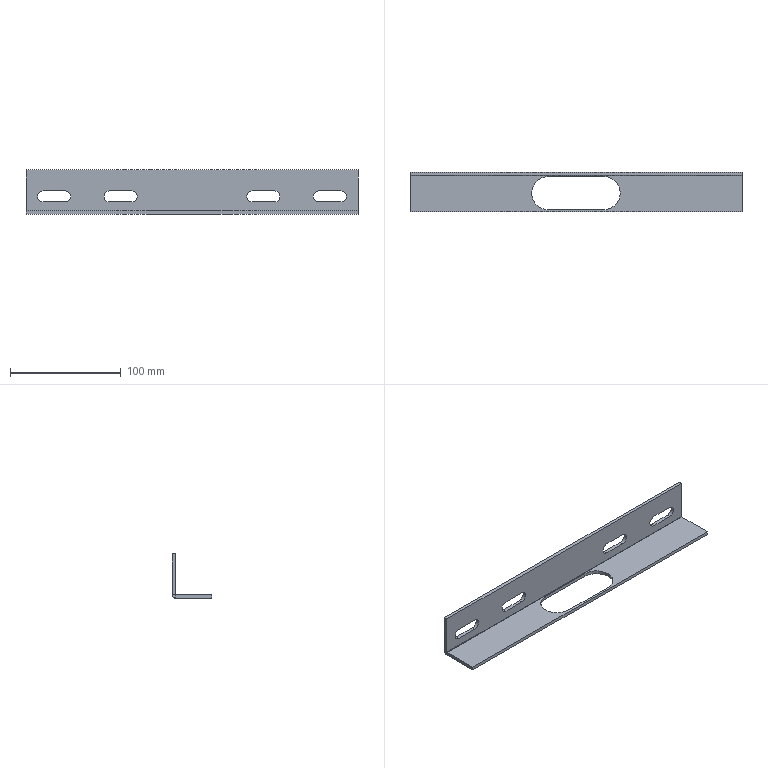Part | SolidWorks | features Cut 2, EdgeFlange 1, FlatPattern 1, SMBaseFlange 1, SheetMetal 1 | 1 solid | 35 faces | box 300 x 36 x 40 mm | volume 55080 mm3 | plane 22 | cylinder 13 | commonest cylinder face diameters 10 x8 30 x3 0.4 x1 6.4 x1
STEP:
#1=CARTESIAN_POINT('',(40.,-1.,-3.));
#2=VERTEX_POINT('',#1);
#3=CARTESIAN_POINT('',(25.,14.,-3.));
#4=VERTEX_POINT('',#3);
#5=CARTESIAN_POINT('',(25.,-1.,-3.));
#6=DIRECTION('',(0.,0.,1.));
#7=DIRECTION('',(1.,0.,0.));
#8=AXIS2_PLACEMENT_3D('',#5,#6,#7);
#9=CIRCLE('',#8,15.);
#10=EDGE_CURVE('',#2,#4,#9,.T.);
#11=ORIENTED_EDGE('',*,*,#10,.F.);
#12=CARTESIAN_POINT('',(40.,-1.,0.));
#13=VERTEX_POINT('',#12);
#14=CARTESIAN_POINT('',(40.,-1.,-10.));
#15=DIRECTION('',(0.,0.,1.));
#16=VECTOR('',#15,1000.);
#17=LINE('',#14,#16);
#18=EDGE_CURVE('',#2,#13,#17,.T.);
#19=ORIENTED_EDGE('',*,*,#18,.T.);
#20=CARTESIAN_POINT('',(25.,14.,0.));
#21=VERTEX_POINT('',#20);
#22=CARTESIAN_POINT('',(25.,-1.,0.));
#23=DIRECTION('',(0.,0.,1.));
#24=DIRECTION('',(1.,0.,0.));
#25=AXIS2_PLACEMENT_3D('',#22,#23,#24);
#26=CIRCLE('',#25,15.);
#27=EDGE_CURVE('',#13,#21,#26,.T.);
#28=ORIENTED_EDGE('',*,*,#27,.T.);
#29=CARTESIAN_POINT('',(25.,14.,-10.));
#30=DIRECTION('',(0.,0.,1.));
#31=VECTOR('',#30,1000.);
#32=LINE('',#29,#31);
#33=EDGE_CURVE('',#4,#21,#32,.T.);
#34=ORIENTED_EDGE('',*,*,#33,.F.);
#35=EDGE_LOOP('',(#11,#19,#28,#34));
#36=FACE_OUTER_BOUND('',#35,.T.);
#37=CARTESIAN_POINT('',(25.,-1.,-10.));
#38=DIRECTION('',(0.,0.,1.));
#39=DIRECTION('',(1.,0.,0.));
#40=AXIS2_PLACEMENT_3D('',#37,#38,#39);
#41=CYLINDRICAL_SURFACE('',#40,15.);
#42=ADVANCED_FACE('',(#36),#41,.F.);
#43=CARTESIAN_POINT('',(-150.,14.8,0.));
#44=VERTEX_POINT('',#43);
#45=CARTESIAN_POINT('',(-150.,-18.,0.));
#46=VERTEX_POINT('',#45);
#47=CARTESIAN_POINT('',(-150.,18.,0.));
#48=DIRECTION('',(0.,-1.,0.));
#49=VECTOR('',#48,1000.);
#50=LINE('',#47,#49);
#51=EDGE_CURVE('',#44,#46,#50,.T.);
#52=ORIENTED_EDGE('',*,*,#51,.F.);
#53=CARTESIAN_POINT('',(-150.,14.8,-3.));
#54=VERTEX_POINT('',#53);
#55=CARTESIAN_POINT('',(-150.,14.8,0.));
#56=DIRECTION('',(0.,0.,-1.));
#57=VECTOR('',#56,1000.);
#58=LINE('',#55,#57);
#59=EDGE_CURVE('',#44,#54,#58,.T.);
#60=ORIENTED_EDGE('',*,*,#59,.T.);
#61=CARTESIAN_POINT('',(-150.,-18.,-3.));
#62=VERTEX_POINT('',#61);
#63=CARTESIAN_POINT('',(-150.,18.,-3.));
#64=DIRECTION('',(0.,-1.,0.));
#65=VECTOR('',#64,1000.);
#66=LINE('',#63,#65);
#67=EDGE_CURVE('',#54,#62,#66,.T.);
#68=ORIENTED_EDGE('',*,*,#67,.T.);
#69=CARTESIAN_POINT('',(-150.,-18.,-3.));
#70=DIRECTION('',(0.,0.,1.));
#71=VECTOR('',#70,1000.);
#72=LINE('',#69,#71);
#73=EDGE_CURVE('',#62,#46,#72,.T.);
#74=ORIENTED_EDGE('',*,*,#73,.T.);
#75=EDGE_LOOP('',(#52,#60,#68,#74));
#76=FACE_OUTER_BOUND('',#75,.T.);
#77=CARTESIAN_POINT('',(-150.,18.,-3.));
#78=DIRECTION('',(-1.,0.,0.));
#79=DIRECTION('',(0.,0.,1.));
#80=AXIS2_PLACEMENT_3D('',#77,#78,#79);
#81=PLANE('',#80);
#82=ADVANCED_FACE('',(#76),#81,.T.);
#83=CARTESIAN_POINT('',(-25.,14.,-3.));
#84=VERTEX_POINT('',#83);
#85=CARTESIAN_POINT('',(0.,14.,-3.));
#86=DIRECTION('',(-1.,0.,0.));
#87=VECTOR('',#86,1000.);
#88=LINE('',#85,#87);
#89=EDGE_CURVE('',#4,#84,#88,.T.);
#90=ORIENTED_EDGE('',*,*,#89,.T.);
#91=CARTESIAN_POINT('',(-25.,-16.,-3.));
#92=VERTEX_POINT('',#91);
#93=CARTESIAN_POINT('',(-25.,-1.,-3.));
#94=DIRECTION('',(0.,0.,1.));
#95=DIRECTION('',(1.,0.,0.));
#96=AXIS2_PLACEMENT_3D('',#93,#94,#95);
#97=CIRCLE('',#96,15.);
#98=EDGE_CURVE('',#84,#92,#97,.T.);
#99=ORIENTED_EDGE('',*,*,#98,.T.);
#100=CARTESIAN_POINT('',(25.,-16.,-3.));
#101=VERTEX_POINT('',#100);
#102=CARTESIAN_POINT('',(0.,-16.,-3.));
#103=DIRECTION('',(1.,0.,0.));
#104=VECTOR('',#103,1000.);
#105=LINE('',#102,#104);
#106=EDGE_CURVE('',#92,#101,#105,.T.);
#107=ORIENTED_EDGE('',*,*,#106,.T.);
#108=CARTESIAN_POINT('',(25.,-1.,-3.));
#109=DIRECTION('',(0.,0.,1.));
#110=DIRECTION('',(1.,0.,0.));
#111=AXIS2_PLACEMENT_3D('',#108,#109,#110);
#112=CIRCLE('',#111,15.);
#113=EDGE_CURVE('',#101,#2,#112,.T.);
#114=ORIENTED_EDGE('',*,*,#113,.T.);
#115=ORIENTED_EDGE('',*,*,#10,.T.);
#116=EDGE_LOOP('',(#90,#99,#107,#114,#115));
#117=FACE_BOUND('',#116,.T.);
#118=CARTESIAN_POINT('',(150.,14.8,-3.));
#119=VERTEX_POINT('',#118);
#120=CARTESIAN_POINT('',(-150.,14.8,-3.));
#121=DIRECTION('',(1.,0.,0.));
#122=VECTOR('',#121,1000.);
#123=LINE('',#120,#122);
#124=EDGE_CURVE('',#54,#119,#123,.T.);
#125=ORIENTED_EDGE('',*,*,#124,.T.);
#126=CARTESIAN_POINT('',(150.,-18.,-3.));
#127=VERTEX_POINT('',#126);
#128=CARTESIAN_POINT('',(150.,18.,-3.));
#129=DIRECTION('',(0.,1.,0.));
#130=VECTOR('',#129,1000.);
#131=LINE('',#128,#130);
#132=EDGE_CURVE('',#127,#119,#131,.T.);
#133=ORIENTED_EDGE('',*,*,#132,.F.);
#134=CARTESIAN_POINT('',(-150.,-18.,-3.));
#135=DIRECTION('',(1.,0.,0.));
#136=VECTOR('',#135,1000.);
#137=LINE('',#134,#136);
#138=EDGE_CURVE('',#62,#127,#137,.T.);
#139=ORIENTED_EDGE('',*,*,#138,.F.);
#140=ORIENTED_EDGE('',*,*,#67,.F.);
#141=EDGE_LOOP('',(#125,#133,#139,#140));
#142=FACE_OUTER_BOUND('',#141,.T.);
#143=CARTESIAN_POINT('',(0.,0.,-3.));
#144=DIRECTION('',(0.,0.,1.));
#145=DIRECTION('',(1.,0.,0.));
#146=AXIS2_PLACEMENT_3D('',#143,#144,#145);
#147=PLANE('',#146);
#148=ADVANCED_FACE('',(#117,#142),#147,.F.);
#149=CARTESIAN_POINT('',(-25.,14.,0.));
#150=VERTEX_POINT('',#149);
#151=CARTESIAN_POINT('',(-25.,-16.,0.));
#152=VERTEX_POINT('',#151);
#153=CARTESIAN_POINT('',(-25.,-1.,0.));
#154=DIRECTION('',(0.,0.,1.));
#155=DIRECTION('',(1.,0.,0.));
#156=AXIS2_PLACEMENT_3D('',#153,#154,#155);
#157=CIRCLE('',#156,15.);
#158=EDGE_CURVE('',#150,#152,#157,.T.);
#159=ORIENTED_EDGE('',*,*,#158,.F.);
#160=CARTESIAN_POINT('',(-25.,14.,0.));
#161=DIRECTION('',(-1.,0.,0.));
#162=VECTOR('',#161,1000.);
#163=LINE('',#160,#162);
#164=EDGE_CURVE('',#21,#150,#163,.T.);
#165=ORIENTED_EDGE('',*,*,#164,.F.);
#166=ORIENTED_EDGE('',*,*,#27,.F.);
#167=CARTESIAN_POINT('',(25.,-16.,0.));
#168=VERTEX_POINT('',#167);
#169=CARTESIAN_POINT('',(25.,-1.,0.));
#170=DIRECTION('',(0.,0.,1.));
#171=DIRECTION('',(1.,0.,0.));
#172=AXIS2_PLACEMENT_3D('',#169,#170,#171);
#173=CIRCLE('',#172,15.);
#174=EDGE_CURVE('',#168,#13,#173,.T.);
#175=ORIENTED_EDGE('',*,*,#174,.F.);
#176=CARTESIAN_POINT('',(-25.,-16.,0.));
#177=DIRECTION('',(1.,0.,0.));
#178=VECTOR('',#177,1000.);
#179=LINE('',#176,#178);
#180=EDGE_CURVE('',#152,#168,#179,.T.);
#181=ORIENTED_EDGE('',*,*,#180,.F.);
#182=EDGE_LOOP('',(#159,#165,#166,#175,#181));
#183=FACE_BOUND('',#182,.T.);
#184=CARTESIAN_POINT('',(150.,-18.,0.));
#185=VERTEX_POINT('',#184);
#186=CARTESIAN_POINT('',(150.,14.8,0.));
#187=VERTEX_POINT('',#186);
#188=CARTESIAN_POINT('',(150.,18.,0.));
#189=DIRECTION('',(0.,1.,0.));
#190=VECTOR('',#189,1000.);
#191=LINE('',#188,#190);
#192=EDGE_CURVE('',#185,#187,#191,.T.);
#193=ORIENTED_EDGE('',*,*,#192,.T.);
#194=CARTESIAN_POINT('',(-150.,14.8,0.));
#195=DIRECTION('',(1.,0.,0.));
#196=VECTOR('',#195,1000.);
#197=LINE('',#194,#196);
#198=EDGE_CURVE('',#44,#187,#197,.T.);
#199=ORIENTED_EDGE('',*,*,#198,.F.);
#200=ORIENTED_EDGE('',*,*,#51,.T.);
#201=CARTESIAN_POINT('',(-150.,-18.,0.));
#202=DIRECTION('',(1.,0.,0.));
#203=VECTOR('',#202,1000.);
#204=LINE('',#201,#203);
#205=EDGE_CURVE('',#46,#185,#204,.T.);
#206=ORIENTED_EDGE('',*,*,#205,.T.);
#207=EDGE_LOOP('',(#193,#199,#200,#206));
#208=FACE_OUTER_BOUND('',#207,.T.);
#209=CARTESIAN_POINT('',(0.,0.,0.));
#210=DIRECTION('',(0.,0.,1.));
#211=DIRECTION('',(1.,0.,0.));
#212=AXIS2_PLACEMENT_3D('',#209,#210,#211);
#213=PLANE('',#212);
#214=ADVANCED_FACE('',(#183,#208),#213,.T.);
#215=CARTESIAN_POINT('',(150.,14.8,0.));
#216=DIRECTION('',(0.,0.,-1.));
#217=VECTOR('',#216,1000.);
#218=LINE('',#215,#217);
#219=EDGE_CURVE('',#187,#119,#218,.T.);
#220=ORIENTED_EDGE('',*,*,#219,.F.);
#221=ORIENTED_EDGE('',*,*,#192,.F.);
#222=CARTESIAN_POINT('',(150.,-18.,-3.));
#223=DIRECTION('',(0.,0.,1.));
#224=VECTOR('',#223,1000.);
#225=LINE('',#222,#224);
#226=EDGE_CURVE('',#127,#185,#225,.T.);
#227=ORIENTED_EDGE('',*,*,#226,.F.);
#228=ORIENTED_EDGE('',*,*,#132,.T.);
#229=EDGE_LOOP('',(#220,#221,#227,#228));
#230=FACE_OUTER_BOUND('',#229,.T.);
#231=CARTESIAN_POINT('',(150.,18.,-3.));
#232=DIRECTION('',(1.,0.,0.));
#233=DIRECTION('',(0.,0.,-1.));
#234=AXIS2_PLACEMENT_3D('',#231,#232,#233);
#235=PLANE('',#234);
#236=ADVANCED_FACE('',(#230),#235,.T.);
#237=ORIENTED_EDGE('',*,*,#205,.F.);
#238=ORIENTED_EDGE('',*,*,#73,.F.);
#239=ORIENTED_EDGE('',*,*,#138,.T.);
#240=ORIENTED_EDGE('',*,*,#226,.T.);
#241=EDGE_LOOP('',(#237,#238,#239,#240));
#242=FACE_OUTER_BOUND('',#241,.T.);
#243=CARTESIAN_POINT('',(-150.,-18.,-3.));
#244=DIRECTION('',(0.,-1.,0.));
#245=DIRECTION('',(0.,0.,-1.));
#246=AXIS2_PLACEMENT_3D('',#243,#244,#245);
#247=PLANE('',#246);
#248=ADVANCED_FACE('',(#242),#247,.T.);
#249=CARTESIAN_POINT('',(150.,15.,0.2));
#250=VERTEX_POINT('',#249);
#251=CARTESIAN_POINT('',(150.,18.,0.2));
#252=VERTEX_POINT('',#251);
#253=CARTESIAN_POINT('',(150.,18.,0.2));
#254=DIRECTION('',(0.,1.,0.));
#255=VECTOR('',#254,1000.);
#256=LINE('',#253,#255);
#257=EDGE_CURVE('',#250,#252,#256,.T.);
#258=ORIENTED_EDGE('',*,*,#257,.F.);
#259=CARTESIAN_POINT('',(150.,14.8,0.2));
#260=DIRECTION('',(1.,0.,0.));
#261=DIRECTION('',(0.,0.,1.));
#262=AXIS2_PLACEMENT_3D('',#259,#260,#261);
#263=CIRCLE('',#262,0.2);
#264=EDGE_CURVE('',#187,#250,#263,.T.);
#265=ORIENTED_EDGE('',*,*,#264,.F.);
#266=ORIENTED_EDGE('',*,*,#219,.T.);
#267=CARTESIAN_POINT('',(150.,14.8,0.2));
#268=DIRECTION('',(1.,0.,0.));
#269=DIRECTION('',(0.,0.,1.));
#270=AXIS2_PLACEMENT_3D('',#267,#268,#269);
#271=CIRCLE('',#270,3.2);
#272=EDGE_CURVE('',#119,#252,#271,.T.);
#273=ORIENTED_EDGE('',*,*,#272,.T.);
#274=EDGE_LOOP('',(#258,#265,#266,#273));
#275=FACE_OUTER_BOUND('',#274,.T.);
#276=CARTESIAN_POINT('',(150.,14.8,0.2));
#277=DIRECTION('',(1.,0.,0.));
#278=DIRECTION('',(0.,0.,-1.));
#279=AXIS2_PLACEMENT_3D('',#276,#277,#278);
#280=PLANE('',#279);
#281=ADVANCED_FACE('',(#275),#280,.T.);
#282=CARTESIAN_POINT('',(-150.,15.,0.2));
#283=VERTEX_POINT('',#282);
#284=CARTESIAN_POINT('',(-150.,14.8,0.2));
#285=DIRECTION('',(-1.,0.,0.));
#286=DIRECTION('',(0.,0.,1.));
#287=AXIS2_PLACEMENT_3D('',#284,#285,#286);
#288=CIRCLE('',#287,0.2);
#289=EDGE_CURVE('',#283,#44,#288,.T.);
#290=ORIENTED_EDGE('',*,*,#289,.F.);
#291=CARTESIAN_POINT('',(-150.,18.,0.2));
#292=VERTEX_POINT('',#291);
#293=CARTESIAN_POINT('',(-150.,15.,0.2));
#294=DIRECTION('',(0.,1.,0.));
#295=VECTOR('',#294,1000.);
#296=LINE('',#293,#295);
#297=EDGE_CURVE('',#283,#292,#296,.T.);
#298=ORIENTED_EDGE('',*,*,#297,.T.);
#299=CARTESIAN_POINT('',(-150.,14.8,0.2));
#300=DIRECTION('',(-1.,0.,0.));
#301=DIRECTION('',(0.,0.,1.));
#302=AXIS2_PLACEMENT_3D('',#299,#300,#301);
#303=CIRCLE('',#302,3.2);
#304=EDGE_CURVE('',#292,#54,#303,.T.);
#305=ORIENTED_EDGE('',*,*,#304,.T.);
#306=ORIENTED_EDGE('',*,*,#59,.F.);
#307=EDGE_LOOP('',(#290,#298,#305,#306));
#308=FACE_OUTER_BOUND('',#307,.T.);
#309=CARTESIAN_POINT('',(-150.,14.8,0.2));
#310=DIRECTION('',(1.,0.,0.));
#311=DIRECTION('',(0.,0.,-1.));
#312=AXIS2_PLACEMENT_3D('',#309,#310,#311);
#313=PLANE('',#312);
#314=ADVANCED_FACE('',(#308),#313,.F.);
#315=ORIENTED_EDGE('',*,*,#124,.F.);
#316=ORIENTED_EDGE('',*,*,#304,.F.);
#317=CARTESIAN_POINT('',(150.,18.,0.2));
#318=DIRECTION('',(1.,0.,0.));
#319=VECTOR('',#318,1000.);
#320=LINE('',#317,#319);
#321=EDGE_CURVE('',#292,#252,#320,.T.);
#322=ORIENTED_EDGE('',*,*,#321,.T.);
#323=ORIENTED_EDGE('',*,*,#272,.F.);
#324=EDGE_LOOP('',(#315,#316,#322,#323));
#325=FACE_OUTER_BOUND('',#324,.T.);
#326=CARTESIAN_POINT('',(-150.,14.8,0.2));
#327=DIRECTION('',(-1.,0.,0.));
#328=DIRECTION('',(0.,1.,0.));
#329=AXIS2_PLACEMENT_3D('',#326,#327,#328);
#330=CYLINDRICAL_SURFACE('',#329,3.2);
#331=ADVANCED_FACE('',(#325),#330,.T.);
#332=ORIENTED_EDGE('',*,*,#198,.T.);
#333=ORIENTED_EDGE('',*,*,#264,.T.);
#334=CARTESIAN_POINT('',(150.,15.,0.2));
#335=DIRECTION('',(-1.,0.,0.));
#336=VECTOR('',#335,1000.);
#337=LINE('',#334,#336);
#338=EDGE_CURVE('',#250,#283,#337,.T.);
#339=ORIENTED_EDGE('',*,*,#338,.T.);
#340=ORIENTED_EDGE('',*,*,#289,.T.);
#341=EDGE_LOOP('',(#332,#333,#339,#340));
#342=FACE_OUTER_BOUND('',#341,.T.);
#343=CARTESIAN_POINT('',(-150.,14.8,0.2));
#344=DIRECTION('',(-1.,0.,0.));
#345=DIRECTION('',(0.,1.,0.));
#346=AXIS2_PLACEMENT_3D('',#343,#344,#345);
#347=CYLINDRICAL_SURFACE('',#346,0.2);
#348=ADVANCED_FACE('',(#342),#347,.F.);
#349=ORIENTED_EDGE('',*,*,#257,.T.);
#350=CARTESIAN_POINT('',(150.,18.,37.));
#351=VERTEX_POINT('',#350);
#352=CARTESIAN_POINT('',(150.,18.,0.));
#353=DIRECTION('',(0.,0.,-1.));
#354=VECTOR('',#353,1000.);
#355=LINE('',#352,#354);
#356=EDGE_CURVE('',#351,#252,#355,.T.);
#357=ORIENTED_EDGE('',*,*,#356,.F.);
#358=CARTESIAN_POINT('',(150.,15.,37.));
#359=VERTEX_POINT('',#358);
#360=CARTESIAN_POINT('',(150.,18.,37.));
#361=DIRECTION('',(0.,-1.,0.));
#362=VECTOR('',#361,1000.);
#363=LINE('',#360,#362);
#364=EDGE_CURVE('',#351,#359,#363,.T.);
#365=ORIENTED_EDGE('',*,*,#364,.T.);
#366=CARTESIAN_POINT('',(150.,15.,0.));
#367=DIRECTION('',(0.,0.,-1.));
#368=VECTOR('',#367,1000.);
#369=LINE('',#366,#368);
#370=EDGE_CURVE('',#359,#250,#369,.T.);
#371=ORIENTED_EDGE('',*,*,#370,.T.);
#372=EDGE_LOOP('',(#349,#357,#365,#371));
#373=FACE_OUTER_BOUND('',#372,.T.);
#374=CARTESIAN_POINT('',(150.,18.,0.));
#375=DIRECTION('',(-1.,0.,0.));
#376=DIRECTION('',(0.,0.,1.));
#377=AXIS2_PLACEMENT_3D('',#374,#375,#376);
#378=PLANE('',#377);
#379=ADVANCED_FACE('',(#373),#378,.F.);
#380=ORIENTED_EDGE('',*,*,#297,.F.);
#381=CARTESIAN_POINT('',(-150.,15.,37.));
#382=VERTEX_POINT('',#381);
#383=CARTESIAN_POINT('',(-150.,15.,37.));
#384=DIRECTION('',(0.,0.,1.));
#385=VECTOR('',#384,1000.);
#386=LINE('',#383,#385);
#387=EDGE_CURVE('',#283,#382,#386,.T.);
#388=ORIENTED_EDGE('',*,*,#387,.T.);
#389=CARTESIAN_POINT('',(-150.,18.,37.));
#390=VERTEX_POINT('',#389);
#391=CARTESIAN_POINT('',(-150.,18.,37.));
#392=DIRECTION('',(0.,-1.,0.));
#393=VECTOR('',#392,1000.);
#394=LINE('',#391,#393);
#395=EDGE_CURVE('',#390,#382,#394,.T.);
#396=ORIENTED_EDGE('',*,*,#395,.F.);
#397=CARTESIAN_POINT('',(-150.,18.,0.));
#398=DIRECTION('',(0.,0.,1.));
#399=VECTOR('',#398,1000.);
#400=LINE('',#397,#399);
#401=EDGE_CURVE('',#292,#390,#400,.T.);
#402=ORIENTED_EDGE('',*,*,#401,.F.);
#403=EDGE_LOOP('',(#380,#388,#396,#402));
#404=FACE_OUTER_BOUND('',#403,.T.);
#405=CARTESIAN_POINT('',(-150.,18.,37.));
#406=DIRECTION('',(1.,0.,0.));
#407=DIRECTION('',(0.,0.,-1.));
#408=AXIS2_PLACEMENT_3D('',#405,#406,#407);
#409=PLANE('',#408);
#410=ADVANCED_FACE('',(#404),#409,.F.);
#411=CARTESIAN_POINT('',(-134.5,18.,18.));
#412=VERTEX_POINT('',#411);
#413=CARTESIAN_POINT('',(-114.5,18.,18.));
#414=VERTEX_POINT('',#413);
#415=CARTESIAN_POINT('',(-134.5,18.,18.));
#416=DIRECTION('',(1.,0.,0.));
#417=VECTOR('',#416,1000.);
#418=LINE('',#415,#417);
#419=EDGE_CURVE('',#412,#414,#418,.T.);
#420=ORIENTED_EDGE('',*,*,#419,.F.);
#421=CARTESIAN_POINT('',(-134.5,18.,8.));
#422=VERTEX_POINT('',#421);
#423=CARTESIAN_POINT('',(-134.5,18.,13.));
#424=DIRECTION('',(0.,1.,0.));
#425=DIRECTION('',(0.,0.,1.));
#426=AXIS2_PLACEMENT_3D('',#423,#424,#425);
#427=CIRCLE('',#426,5.);
#428=EDGE_CURVE('',#422,#412,#427,.T.);
#429=ORIENTED_EDGE('',*,*,#428,.F.);
#430=CARTESIAN_POINT('',(-114.5,18.,8.));
#431=VERTEX_POINT('',#430);
#432=CARTESIAN_POINT('',(-134.5,18.,8.));
#433=DIRECTION('',(-1.,0.,0.));
#434=VECTOR('',#433,1000.);
#435=LINE('',#432,#434);
#436=EDGE_CURVE('',#431,#422,#435,.T.);
#437=ORIENTED_EDGE('',*,*,#436,.F.);
#438=CARTESIAN_POINT('',(-114.5,18.,13.));
#439=DIRECTION('',(0.,1.,0.));
#440=DIRECTION('',(0.,0.,1.));
#441=AXIS2_PLACEMENT_3D('',#438,#439,#440);
#442=CIRCLE('',#441,5.);
#443=EDGE_CURVE('',#414,#431,#442,.T.);
#444=ORIENTED_EDGE('',*,*,#443,.F.);
#445=EDGE_LOOP('',(#420,#429,#437,#444));
#446=FACE_BOUND('',#445,.T.);
#447=CARTESIAN_POINT('',(-74.5,18.,18.));
#448=VERTEX_POINT('',#447);
#449=CARTESIAN_POINT('',(-54.5,18.,18.));
#450=VERTEX_POINT('',#449);
#451=CARTESIAN_POINT('',(-74.5,18.,18.));
#452=DIRECTION('',(1.,0.,0.));
#453=VECTOR('',#452,1000.);
#454=LINE('',#451,#453);
#455=EDGE_CURVE('',#448,#450,#454,.T.);
#456=ORIENTED_EDGE('',*,*,#455,.F.);
#457=CARTESIAN_POINT('',(-74.5,18.,8.));
#458=VERTEX_POINT('',#457);
#459=CARTESIAN_POINT('',(-74.5,18.,13.));
#460=DIRECTION('',(0.,1.,0.));
#461=DIRECTION('',(0.,0.,1.));
#462=AXIS2_PLACEMENT_3D('',#459,#460,#461);
#463=CIRCLE('',#462,5.);
#464=EDGE_CURVE('',#458,#448,#463,.T.);
#465=ORIENTED_EDGE('',*,*,#464,.F.);
#466=CARTESIAN_POINT('',(-54.5,18.,8.));
#467=VERTEX_POINT('',#466);
#468=CARTESIAN_POINT('',(-74.5,18.,8.));
#469=DIRECTION('',(-1.,0.,0.));
#470=VECTOR('',#469,1000.);
#471=LINE('',#468,#470);
#472=EDGE_CURVE('',#467,#458,#471,.T.);
#473=ORIENTED_EDGE('',*,*,#472,.F.);
#474=CARTESIAN_POINT('',(-54.5,18.,13.));
#475=DIRECTION('',(0.,1.,0.));
#476=DIRECTION('',(0.,0.,1.));
#477=AXIS2_PLACEMENT_3D('',#474,#475,#476);
#478=CIRCLE('',#477,5.);
#479=EDGE_CURVE('',#450,#467,#478,.T.);
#480=ORIENTED_EDGE('',*,*,#479,.F.);
#481=EDGE_LOOP('',(#456,#465,#473,#480));
#482=FACE_BOUND('',#481,.T.);
#483=CARTESIAN_POINT('',(74.5,18.,8.));
#484=VERTEX_POINT('',#483);
#485=CARTESIAN_POINT('',(54.5,18.,8.));
#486=VERTEX_POINT('',#485);
#487=CARTESIAN_POINT('',(74.5,18.,8.));
#488=DIRECTION('',(-1.,0.,0.));
#489=VECTOR('',#488,1000.);
#490=LINE('',#487,#489);
#491=EDGE_CURVE('',#484,#486,#490,.T.);
#492=ORIENTED_EDGE('',*,*,#491,.F.);
#493=CARTESIAN_POINT('',(74.5,18.,18.));
#494=VERTEX_POINT('',#493);
#495=CARTESIAN_POINT('',(74.5,18.,13.));
#496=DIRECTION('',(0.,1.,0.));
#497=DIRECTION('',(0.,0.,-1.));
#498=AXIS2_PLACEMENT_3D('',#495,#496,#497);
#499=CIRCLE('',#498,5.);
#500=EDGE_CURVE('',#494,#484,#499,.T.);
#501=ORIENTED_EDGE('',*,*,#500,.F.);
#502=CARTESIAN_POINT('',(54.5,18.,18.));
#503=VERTEX_POINT('',#502);
#504=CARTESIAN_POINT('',(74.5,18.,18.));
#505=DIRECTION('',(1.,0.,0.));
#506=VECTOR('',#505,1000.);
#507=LINE('',#504,#506);
#508=EDGE_CURVE('',#503,#494,#507,.T.);
#509=ORIENTED_EDGE('',*,*,#508,.F.);
#510=CARTESIAN_POINT('',(54.5,18.,13.));
#511=DIRECTION('',(0.,1.,0.));
#512=DIRECTION('',(0.,0.,-1.));
#513=AXIS2_PLACEMENT_3D('',#510,#511,#512);
#514=CIRCLE('',#513,5.);
#515=EDGE_CURVE('',#486,#503,#514,.T.);
#516=ORIENTED_EDGE('',*,*,#515,.F.);
#517=EDGE_LOOP('',(#492,#501,#509,#516));
#518=FACE_BOUND('',#517,.T.);
#519=CARTESIAN_POINT('',(134.5,18.,8.));
#520=VERTEX_POINT('',#519);
#521=CARTESIAN_POINT('',(114.5,18.,8.));
#522=VERTEX_POINT('',#521);
#523=CARTESIAN_POINT('',(134.5,18.,8.));
#524=DIRECTION('',(-1.,0.,0.));
#525=VECTOR('',#524,1000.);
#526=LINE('',#523,#525);
#527=EDGE_CURVE('',#520,#522,#526,.T.);
#528=ORIENTED_EDGE('',*,*,#527,.F.);
#529=CARTESIAN_POINT('',(134.5,18.,18.));
#530=VERTEX_POINT('',#529);
#531=CARTESIAN_POINT('',(134.5,18.,13.));
#532=DIRECTION('',(0.,1.,0.));
#533=DIRECTION('',(0.,0.,-1.));
#534=AXIS2_PLACEMENT_3D('',#531,#532,#533);
#535=CIRCLE('',#534,5.);
#536=EDGE_CURVE('',#530,#520,#535,.T.);
#537=ORIENTED_EDGE('',*,*,#536,.F.);
#538=CARTESIAN_POINT('',(114.5,18.,18.));
#539=VERTEX_POINT('',#538);
#540=CARTESIAN_POINT('',(134.5,18.,18.));
#541=DIRECTION('',(1.,0.,0.));
#542=VECTOR('',#541,1000.);
#543=LINE('',#540,#542);
#544=EDGE_CURVE('',#539,#530,#543,.T.);
#545=ORIENTED_EDGE('',*,*,#544,.F.);
#546=CARTESIAN_POINT('',(114.5,18.,13.));
#547=DIRECTION('',(0.,1.,0.));
#548=DIRECTION('',(0.,0.,-1.));
#549=AXIS2_PLACEMENT_3D('',#546,#547,#548);
#550=CIRCLE('',#549,5.);
#551=EDGE_CURVE('',#522,#539,#550,.T.);
#552=ORIENTED_EDGE('',*,*,#551,.F.);
#553=EDGE_LOOP('',(#528,#537,#545,#552));
#554=FACE_BOUND('',#553,.T.);
#555=ORIENTED_EDGE('',*,*,#321,.F.);
#556=ORIENTED_EDGE('',*,*,#401,.T.);
#557=CARTESIAN_POINT('',(0.,18.,37.));
#558=DIRECTION('',(1.,0.,0.));
#559=VECTOR('',#558,1000.);
#560=LINE('',#557,#559);
#561=EDGE_CURVE('',#390,#351,#560,.T.);
#562=ORIENTED_EDGE('',*,*,#561,.T.);
#563=ORIENTED_EDGE('',*,*,#356,.T.);
#564=EDGE_LOOP('',(#555,#556,#562,#563));
#565=FACE_OUTER_BOUND('',#564,.T.);
#566=CARTESIAN_POINT('',(0.,18.,0.));
#567=DIRECTION('',(0.,-1.,0.));
#568=DIRECTION('',(0.,0.,-1.));
#569=AXIS2_PLACEMENT_3D('',#566,#567,#568);
#570=PLANE('',#569);
#571=ADVANCED_FACE('',(#446,#482,#518,#554,#565),#570,.F.);
#572=CARTESIAN_POINT('',(-134.5,15.,18.));
#573=VERTEX_POINT('',#572);
#574=CARTESIAN_POINT('',(-134.5,15.,8.));
#575=VERTEX_POINT('',#574);
#576=CARTESIAN_POINT('',(-134.5,15.,13.));
#577=DIRECTION('',(0.,-1.,0.));
#578=DIRECTION('',(0.,0.,-1.));
#579=AXIS2_PLACEMENT_3D('',#576,#577,#578);
#580=CIRCLE('',#579,5.);
#581=EDGE_CURVE('',#573,#575,#580,.T.);
#582=ORIENTED_EDGE('',*,*,#581,.F.);
#583=CARTESIAN_POINT('',(-114.5,15.,18.));
#584=VERTEX_POINT('',#583);
#585=CARTESIAN_POINT('',(0.,15.,18.));
#586=DIRECTION('',(-1.,0.,0.));
#587=VECTOR('',#586,1000.);
#588=LINE('',#585,#587);
#589=EDGE_CURVE('',#584,#573,#588,.T.);
#590=ORIENTED_EDGE('',*,*,#589,.F.);
#591=CARTESIAN_POINT('',(-114.5,15.,8.));
#592=VERTEX_POINT('',#591);
#593=CARTESIAN_POINT('',(-114.5,15.,13.));
#594=DIRECTION('',(0.,-1.,0.));
#595=DIRECTION('',(0.,0.,-1.));
#596=AXIS2_PLACEMENT_3D('',#593,#594,#595);
#597=CIRCLE('',#596,5.);
#598=EDGE_CURVE('',#592,#584,#597,.T.);
#599=ORIENTED_EDGE('',*,*,#598,.F.);
#600=CARTESIAN_POINT('',(0.,15.,8.));
#601=DIRECTION('',(1.,0.,0.));
#602=VECTOR('',#601,1000.);
#603=LINE('',#600,#602);
#604=EDGE_CURVE('',#575,#592,#603,.T.);
#605=ORIENTED_EDGE('',*,*,#604,.F.);
#606=EDGE_LOOP('',(#582,#590,#599,#605));
#607=FACE_BOUND('',#606,.T.);
#608=CARTESIAN_POINT('',(-74.5,15.,18.));
#609=VERTEX_POINT('',#608);
#610=CARTESIAN_POINT('',(-74.5,15.,8.));
#611=VERTEX_POINT('',#610);
#612=CARTESIAN_POINT('',(-74.5,15.,13.));
#613=DIRECTION('',(0.,-1.,0.));
#614=DIRECTION('',(0.,0.,-1.));
#615=AXIS2_PLACEMENT_3D('',#612,#613,#614);
#616=CIRCLE('',#615,5.);
#617=EDGE_CURVE('',#609,#611,#616,.T.);
#618=ORIENTED_EDGE('',*,*,#617,.F.);
#619=CARTESIAN_POINT('',(-54.5,15.,18.));
#620=VERTEX_POINT('',#619);
#621=CARTESIAN_POINT('',(0.,15.,18.));
#622=DIRECTION('',(-1.,0.,0.));
#623=VECTOR('',#622,1000.);
#624=LINE('',#621,#623);
#625=EDGE_CURVE('',#620,#609,#624,.T.);
#626=ORIENTED_EDGE('',*,*,#625,.F.);
#627=CARTESIAN_POINT('',(-54.5,15.,8.));
#628=VERTEX_POINT('',#627);
#629=CARTESIAN_POINT('',(-54.5,15.,13.));
#630=DIRECTION('',(0.,-1.,0.));
#631=DIRECTION('',(0.,0.,-1.));
#632=AXIS2_PLACEMENT_3D('',#629,#630,#631);
#633=CIRCLE('',#632,5.);
#634=EDGE_CURVE('',#628,#620,#633,.T.);
#635=ORIENTED_EDGE('',*,*,#634,.F.);
#636=CARTESIAN_POINT('',(0.,15.,8.));
#637=DIRECTION('',(1.,0.,0.));
#638=VECTOR('',#637,1000.);
#639=LINE('',#636,#638);
#640=EDGE_CURVE('',#611,#628,#639,.T.);
#641=ORIENTED_EDGE('',*,*,#640,.F.);
#642=EDGE_LOOP('',(#618,#626,#635,#641));
#643=FACE_BOUND('',#642,.T.);
#644=CARTESIAN_POINT('',(74.5,15.,8.));
#645=VERTEX_POINT('',#644);
#646=CARTESIAN_POINT('',(74.5,15.,18.));
#647=VERTEX_POINT('',#646);
#648=CARTESIAN_POINT('',(74.5,15.,13.));
#649=DIRECTION('',(0.,-1.,0.));
#650=DIRECTION('',(0.,0.,-1.));
#651=AXIS2_PLACEMENT_3D('',#648,#649,#650);
#652=CIRCLE('',#651,5.);
#653=EDGE_CURVE('',#645,#647,#652,.T.);
#654=ORIENTED_EDGE('',*,*,#653,.F.);
#655=CARTESIAN_POINT('',(54.5,15.,8.));
#656=VERTEX_POINT('',#655);
#657=CARTESIAN_POINT('',(0.,15.,8.));
#658=DIRECTION('',(1.,0.,0.));
#659=VECTOR('',#658,1000.);
#660=LINE('',#657,#659);
#661=EDGE_CURVE('',#656,#645,#660,.T.);
#662=ORIENTED_EDGE('',*,*,#661,.F.);
#663=CARTESIAN_POINT('',(54.5,15.,18.));
#664=VERTEX_POINT('',#663);
#665=CARTESIAN_POINT('',(54.5,15.,13.));
#666=DIRECTION('',(0.,-1.,0.));
#667=DIRECTION('',(0.,0.,-1.));
#668=AXIS2_PLACEMENT_3D('',#665,#666,#667);
#669=CIRCLE('',#668,5.);
#670=EDGE_CURVE('',#664,#656,#669,.T.);
#671=ORIENTED_EDGE('',*,*,#670,.F.);
#672=CARTESIAN_POINT('',(0.,15.,18.));
#673=DIRECTION('',(-1.,0.,0.));
#674=VECTOR('',#673,1000.);
#675=LINE('',#672,#674);
#676=EDGE_CURVE('',#647,#664,#675,.T.);
#677=ORIENTED_EDGE('',*,*,#676,.F.);
#678=EDGE_LOOP('',(#654,#662,#671,#677));
#679=FACE_BOUND('',#678,.T.);
#680=CARTESIAN_POINT('',(134.5,15.,8.));
#681=VERTEX_POINT('',#680);
#682=CARTESIAN_POINT('',(134.5,15.,18.));
#683=VERTEX_POINT('',#682);
#684=CARTESIAN_POINT('',(134.5,15.,13.));
#685=DIRECTION('',(0.,-1.,0.));
#686=DIRECTION('',(0.,0.,-1.));
#687=AXIS2_PLACEMENT_3D('',#684,#685,#686);
#688=CIRCLE('',#687,5.);
#689=EDGE_CURVE('',#681,#683,#688,.T.);
#690=ORIENTED_EDGE('',*,*,#689,.F.);
#691=CARTESIAN_POINT('',(114.5,15.,8.));
#692=VERTEX_POINT('',#691);
#693=CARTESIAN_POINT('',(0.,15.,8.));
#694=DIRECTION('',(1.,0.,0.));
#695=VECTOR('',#694,1000.);
#696=LINE('',#693,#695);
#697=EDGE_CURVE('',#692,#681,#696,.T.);
#698=ORIENTED_EDGE('',*,*,#697,.F.);
#699=CARTESIAN_POINT('',(114.5,15.,18.));
#700=VERTEX_POINT('',#699);
#701=CARTESIAN_POINT('',(114.5,15.,13.));
#702=DIRECTION('',(0.,-1.,0.));
#703=DIRECTION('',(0.,0.,-1.));
#704=AXIS2_PLACEMENT_3D('',#701,#702,#703);
#705=CIRCLE('',#704,5.);
#706=EDGE_CURVE('',#700,#692,#705,.T.);
#707=ORIENTED_EDGE('',*,*,#706,.F.);
#708=CARTESIAN_POINT('',(0.,15.,18.));
#709=DIRECTION('',(-1.,0.,0.));
#710=VECTOR('',#709,1000.);
#711=LINE('',#708,#710);
#712=EDGE_CURVE('',#683,#700,#711,.T.);
#713=ORIENTED_EDGE('',*,*,#712,.F.);
#714=EDGE_LOOP('',(#690,#698,#707,#713));
#715=FACE_BOUND('',#714,.T.);
#716=ORIENTED_EDGE('',*,*,#387,.F.);
#717=ORIENTED_EDGE('',*,*,#338,.F.);
#718=ORIENTED_EDGE('',*,*,#370,.F.);
#719=CARTESIAN_POINT('',(150.,15.,37.));
#720=DIRECTION('',(1.,0.,0.));
#721=VECTOR('',#720,1000.);
#722=LINE('',#719,#721);
#723=EDGE_CURVE('',#382,#359,#722,.T.);
#724=ORIENTED_EDGE('',*,*,#723,.F.);
#725=EDGE_LOOP('',(#716,#717,#718,#724));
#726=FACE_OUTER_BOUND('',#725,.T.);
#727=CARTESIAN_POINT('',(0.,15.,0.));
#728=DIRECTION('',(0.,-1.,0.));
#729=DIRECTION('',(0.,0.,-1.));
#730=AXIS2_PLACEMENT_3D('',#727,#728,#729);
#731=PLANE('',#730);
#732=ADVANCED_FACE('',(#607,#643,#679,#715,#726),#731,.T.);
#733=ORIENTED_EDGE('',*,*,#723,.T.);
#734=ORIENTED_EDGE('',*,*,#364,.F.);
#735=ORIENTED_EDGE('',*,*,#561,.F.);
#736=ORIENTED_EDGE('',*,*,#395,.T.);
#737=EDGE_LOOP('',(#733,#734,#735,#736));
#738=FACE_OUTER_BOUND('',#737,.T.);
#739=CARTESIAN_POINT('',(150.,18.,37.));
#740=DIRECTION('',(0.,0.,-1.));
#741=DIRECTION('',(0.,1.,0.));
#742=AXIS2_PLACEMENT_3D('',#739,#740,#741);
#743=PLANE('',#742);
#744=ADVANCED_FACE('',(#738),#743,.F.);
#745=CARTESIAN_POINT('',(-25.,14.,-10.));
#746=DIRECTION('',(0.,0.,1.));
#747=VECTOR('',#746,1000.);
#748=LINE('',#745,#747);
#749=EDGE_CURVE('',#84,#150,#748,.T.);
#750=ORIENTED_EDGE('',*,*,#749,.T.);
#751=ORIENTED_EDGE('',*,*,#158,.T.);
#752=CARTESIAN_POINT('',(-25.,-16.,-10.));
#753=DIRECTION('',(0.,0.,1.));
#754=VECTOR('',#753,1000.);
#755=LINE('',#752,#754);
#756=EDGE_CURVE('',#92,#152,#755,.T.);
#757=ORIENTED_EDGE('',*,*,#756,.F.);
#758=ORIENTED_EDGE('',*,*,#98,.F.);
#759=EDGE_LOOP('',(#750,#751,#757,#758));
#760=FACE_OUTER_BOUND('',#759,.T.);
#761=CARTESIAN_POINT('',(-25.,-1.,-10.));
#762=DIRECTION('',(0.,0.,1.));
#763=DIRECTION('',(1.,0.,0.));
#764=AXIS2_PLACEMENT_3D('',#761,#762,#763);
#765=CYLINDRICAL_SURFACE('',#764,15.);
#766=ADVANCED_FACE('',(#760),#765,.F.);
#767=ORIENTED_EDGE('',*,*,#33,.T.);
#768=ORIENTED_EDGE('',*,*,#164,.T.);
#769=ORIENTED_EDGE('',*,*,#749,.F.);
#770=ORIENTED_EDGE('',*,*,#89,.F.);
#771=EDGE_LOOP('',(#767,#768,#769,#770));
#772=FACE_OUTER_BOUND('',#771,.T.);
#773=CARTESIAN_POINT('',(-25.,14.,-10.));
#774=DIRECTION('',(0.,1.,0.));
#775=DIRECTION('',(-1.,0.,0.));
#776=AXIS2_PLACEMENT_3D('',#773,#774,#775);
#777=PLANE('',#776);
#778=ADVANCED_FACE('',(#772),#777,.F.);
#779=ORIENTED_EDGE('',*,*,#18,.F.);
#780=ORIENTED_EDGE('',*,*,#113,.F.);
#781=CARTESIAN_POINT('',(25.,-16.,-10.));
#782=DIRECTION('',(0.,0.,1.));
#783=VECTOR('',#782,1000.);
#784=LINE('',#781,#783);
#785=EDGE_CURVE('',#101,#168,#784,.T.);
#786=ORIENTED_EDGE('',*,*,#785,.T.);
#787=ORIENTED_EDGE('',*,*,#174,.T.);
#788=EDGE_LOOP('',(#779,#780,#786,#787));
#789=FACE_OUTER_BOUND('',#788,.T.);
#790=CARTESIAN_POINT('',(25.,-1.,-10.));
#791=DIRECTION('',(0.,0.,1.));
#792=DIRECTION('',(1.,0.,0.));
#793=AXIS2_PLACEMENT_3D('',#790,#791,#792);
#794=CYLINDRICAL_SURFACE('',#793,15.);
#795=ADVANCED_FACE('',(#789),#794,.F.);
#796=ORIENTED_EDGE('',*,*,#756,.T.);
#797=ORIENTED_EDGE('',*,*,#180,.T.);
#798=ORIENTED_EDGE('',*,*,#785,.F.);
#799=ORIENTED_EDGE('',*,*,#106,.F.);
#800=EDGE_LOOP('',(#796,#797,#798,#799));
#801=FACE_OUTER_BOUND('',#800,.T.);
#802=CARTESIAN_POINT('',(-25.,-16.,-10.));
#803=DIRECTION('',(0.,-1.,0.));
#804=DIRECTION('',(1.,0.,0.));
#805=AXIS2_PLACEMENT_3D('',#802,#803,#804);
#806=PLANE('',#805);
#807=ADVANCED_FACE('',(#801),#806,.F.);
#808=ORIENTED_EDGE('',*,*,#689,.T.);
#809=CARTESIAN_POINT('',(134.5,8.,18.));
#810=DIRECTION('',(0.,1.,0.));
#811=VECTOR('',#810,1000.);
#812=LINE('',#809,#811);
#813=EDGE_CURVE('',#683,#530,#812,.T.);
#814=ORIENTED_EDGE('',*,*,#813,.T.);
#815=ORIENTED_EDGE('',*,*,#536,.T.);
#816=CARTESIAN_POINT('',(134.5,8.,8.));
#817=DIRECTION('',(0.,1.,0.));
#818=VECTOR('',#817,1000.);
#819=LINE('',#816,#818);
#820=EDGE_CURVE('',#681,#520,#819,.T.);
#821=ORIENTED_EDGE('',*,*,#820,.F.);
#822=EDGE_LOOP('',(#808,#814,#815,#821));
#823=FACE_OUTER_BOUND('',#822,.T.);
#824=CARTESIAN_POINT('',(134.5,8.,13.));
#825=DIRECTION('',(0.,1.,0.));
#826=DIRECTION('',(0.,0.,1.));
#827=AXIS2_PLACEMENT_3D('',#824,#825,#826);
#828=CYLINDRICAL_SURFACE('',#827,5.);
#829=ADVANCED_FACE('',(#823),#828,.F.);
#830=ORIENTED_EDGE('',*,*,#712,.T.);
#831=CARTESIAN_POINT('',(114.5,8.,18.));
#832=DIRECTION('',(0.,1.,0.));
#833=VECTOR('',#832,1000.);
#834=LINE('',#831,#833);
#835=EDGE_CURVE('',#700,#539,#834,.T.);
#836=ORIENTED_EDGE('',*,*,#835,.T.);
#837=ORIENTED_EDGE('',*,*,#544,.T.);
#838=ORIENTED_EDGE('',*,*,#813,.F.);
#839=EDGE_LOOP('',(#830,#836,#837,#838));
#840=FACE_OUTER_BOUND('',#839,.T.);
#841=CARTESIAN_POINT('',(134.5,8.,18.));
#842=DIRECTION('',(0.,0.,1.));
#843=DIRECTION('',(0.,-1.,0.));
#844=AXIS2_PLACEMENT_3D('',#841,#842,#843);
#845=PLANE('',#844);
#846=ADVANCED_FACE('',(#840),#845,.F.);
#847=ORIENTED_EDGE('',*,*,#706,.T.);
#848=CARTESIAN_POINT('',(114.5,8.,8.));
#849=DIRECTION('',(0.,1.,0.));
#850=VECTOR('',#849,1000.);
#851=LINE('',#848,#850);
#852=EDGE_CURVE('',#692,#522,#851,.T.);
#853=ORIENTED_EDGE('',*,*,#852,.T.);
#854=ORIENTED_EDGE('',*,*,#551,.T.);
#855=ORIENTED_EDGE('',*,*,#835,.F.);
#856=EDGE_LOOP('',(#847,#853,#854,#855));
#857=FACE_OUTER_BOUND('',#856,.T.);
#858=CARTESIAN_POINT('',(114.5,8.,13.));
#859=DIRECTION('',(0.,1.,0.));
#860=DIRECTION('',(0.,0.,1.));
#861=AXIS2_PLACEMENT_3D('',#858,#859,#860);
#862=CYLINDRICAL_SURFACE('',#861,5.);
#863=ADVANCED_FACE('',(#857),#862,.F.);
#864=ORIENTED_EDGE('',*,*,#697,.T.);
#865=ORIENTED_EDGE('',*,*,#820,.T.);
#866=ORIENTED_EDGE('',*,*,#527,.T.);
#867=ORIENTED_EDGE('',*,*,#852,.F.);
#868=EDGE_LOOP('',(#864,#865,#866,#867));
#869=FACE_OUTER_BOUND('',#868,.T.);
#870=CARTESIAN_POINT('',(134.5,8.,8.));
#871=DIRECTION('',(0.,0.,-1.));
#872=DIRECTION('',(0.,1.,0.));
#873=AXIS2_PLACEMENT_3D('',#870,#871,#872);
#874=PLANE('',#873);
#875=ADVANCED_FACE('',(#869),#874,.F.);
#876=ORIENTED_EDGE('',*,*,#653,.T.);
#877=CARTESIAN_POINT('',(74.5,8.,18.));
#878=DIRECTION('',(0.,1.,0.));
#879=VECTOR('',#878,1000.);
#880=LINE('',#877,#879);
#881=EDGE_CURVE('',#647,#494,#880,.T.);
#882=ORIENTED_EDGE('',*,*,#881,.T.);
#883=ORIENTED_EDGE('',*,*,#500,.T.);
#884=CARTESIAN_POINT('',(74.5,8.,8.));
#885=DIRECTION('',(0.,1.,0.));
#886=VECTOR('',#885,1000.);
#887=LINE('',#884,#886);
#888=EDGE_CURVE('',#645,#484,#887,.T.);
#889=ORIENTED_EDGE('',*,*,#888,.F.);
#890=EDGE_LOOP('',(#876,#882,#883,#889));
#891=FACE_OUTER_BOUND('',#890,.T.);
#892=CARTESIAN_POINT('',(74.5,8.,13.));
#893=DIRECTION('',(0.,1.,0.));
#894=DIRECTION('',(0.,0.,1.));
#895=AXIS2_PLACEMENT_3D('',#892,#893,#894);
#896=CYLINDRICAL_SURFACE('',#895,5.);
#897=ADVANCED_FACE('',(#891),#896,.F.);
#898=ORIENTED_EDGE('',*,*,#676,.T.);
#899=CARTESIAN_POINT('',(54.5,8.,18.));
#900=DIRECTION('',(0.,1.,0.));
#901=VECTOR('',#900,1000.);
#902=LINE('',#899,#901);
#903=EDGE_CURVE('',#664,#503,#902,.T.);
#904=ORIENTED_EDGE('',*,*,#903,.T.);
#905=ORIENTED_EDGE('',*,*,#508,.T.);
#906=ORIENTED_EDGE('',*,*,#881,.F.);
#907=EDGE_LOOP('',(#898,#904,#905,#906));
#908=FACE_OUTER_BOUND('',#907,.T.);
#909=CARTESIAN_POINT('',(74.5,8.,18.));
#910=DIRECTION('',(0.,0.,1.));
#911=DIRECTION('',(0.,-1.,0.));
#912=AXIS2_PLACEMENT_3D('',#909,#910,#911);
#913=PLANE('',#912);
#914=ADVANCED_FACE('',(#908),#913,.F.);
#915=ORIENTED_EDGE('',*,*,#670,.T.);
#916=CARTESIAN_POINT('',(54.5,8.,8.));
#917=DIRECTION('',(0.,1.,0.));
#918=VECTOR('',#917,1000.);
#919=LINE('',#916,#918);
#920=EDGE_CURVE('',#656,#486,#919,.T.);
#921=ORIENTED_EDGE('',*,*,#920,.T.);
#922=ORIENTED_EDGE('',*,*,#515,.T.);
#923=ORIENTED_EDGE('',*,*,#903,.F.);
#924=EDGE_LOOP('',(#915,#921,#922,#923));
#925=FACE_OUTER_BOUND('',#924,.T.);
#926=CARTESIAN_POINT('',(54.5,8.,13.));
#927=DIRECTION('',(0.,1.,0.));
#928=DIRECTION('',(0.,0.,1.));
#929=AXIS2_PLACEMENT_3D('',#926,#927,#928);
#930=CYLINDRICAL_SURFACE('',#929,5.);
#931=ADVANCED_FACE('',(#925),#930,.F.);
#932=ORIENTED_EDGE('',*,*,#661,.T.);
#933=ORIENTED_EDGE('',*,*,#888,.T.);
#934=ORIENTED_EDGE('',*,*,#491,.T.);
#935=ORIENTED_EDGE('',*,*,#920,.F.);
#936=EDGE_LOOP('',(#932,#933,#934,#935));
#937=FACE_OUTER_BOUND('',#936,.T.);
#938=CARTESIAN_POINT('',(74.5,8.,8.));
#939=DIRECTION('',(0.,0.,-1.));
#940=DIRECTION('',(0.,1.,0.));
#941=AXIS2_PLACEMENT_3D('',#938,#939,#940);
#942=PLANE('',#941);
#943=ADVANCED_FACE('',(#937),#942,.F.);
#944=ORIENTED_EDGE('',*,*,#617,.T.);
#945=CARTESIAN_POINT('',(-74.5,8.,8.));
#946=DIRECTION('',(0.,1.,0.));
#947=VECTOR('',#946,1000.);
#948=LINE('',#945,#947);
#949=EDGE_CURVE('',#611,#458,#948,.T.);
#950=ORIENTED_EDGE('',*,*,#949,.T.);
#951=ORIENTED_EDGE('',*,*,#464,.T.);
#952=CARTESIAN_POINT('',(-74.5,8.,18.));
#953=DIRECTION('',(0.,1.,0.));
#954=VECTOR('',#953,1000.);
#955=LINE('',#952,#954);
#956=EDGE_CURVE('',#609,#448,#955,.T.);
#957=ORIENTED_EDGE('',*,*,#956,.F.);
#958=EDGE_LOOP('',(#944,#950,#951,#957));
#959=FACE_OUTER_BOUND('',#958,.T.);
#960=CARTESIAN_POINT('',(-74.5,8.,13.));
#961=DIRECTION('',(0.,1.,0.));
#962=DIRECTION('',(0.,0.,1.));
#963=AXIS2_PLACEMENT_3D('',#960,#961,#962);
#964=CYLINDRICAL_SURFACE('',#963,5.);
#965=ADVANCED_FACE('',(#959),#964,.F.);
#966=ORIENTED_EDGE('',*,*,#640,.T.);
#967=CARTESIAN_POINT('',(-54.5,8.,8.));
#968=DIRECTION('',(0.,1.,0.));
#969=VECTOR('',#968,1000.);
#970=LINE('',#967,#969);
#971=EDGE_CURVE('',#628,#467,#970,.T.);
#972=ORIENTED_EDGE('',*,*,#971,.T.);
#973=ORIENTED_EDGE('',*,*,#472,.T.);
#974=ORIENTED_EDGE('',*,*,#949,.F.);
#975=EDGE_LOOP('',(#966,#972,#973,#974));
#976=FACE_OUTER_BOUND('',#975,.T.);
#977=CARTESIAN_POINT('',(-74.5,8.,8.));
#978=DIRECTION('',(0.,0.,-1.));
#979=DIRECTION('',(0.,1.,0.));
#980=AXIS2_PLACEMENT_3D('',#977,#978,#979);
#981=PLANE('',#980);
#982=ADVANCED_FACE('',(#976),#981,.F.);
#983=ORIENTED_EDGE('',*,*,#634,.T.);
#984=CARTESIAN_POINT('',(-54.5,8.,18.));
#985=DIRECTION('',(0.,1.,0.));
#986=VECTOR('',#985,1000.);
#987=LINE('',#984,#986);
#988=EDGE_CURVE('',#620,#450,#987,.T.);
#989=ORIENTED_EDGE('',*,*,#988,.T.);
#990=ORIENTED_EDGE('',*,*,#479,.T.);
#991=ORIENTED_EDGE('',*,*,#971,.F.);
#992=EDGE_LOOP('',(#983,#989,#990,#991));
#993=FACE_OUTER_BOUND('',#992,.T.);
#994=CARTESIAN_POINT('',(-54.5,8.,13.));
#995=DIRECTION('',(0.,1.,0.));
#996=DIRECTION('',(0.,0.,1.));
#997=AXIS2_PLACEMENT_3D('',#994,#995,#996);
#998=CYLINDRICAL_SURFACE('',#997,5.);
#999=ADVANCED_FACE('',(#993),#998,.F.);
#1000=ORIENTED_EDGE('',*,*,#625,.T.);
#1001=ORIENTED_EDGE('',*,*,#956,.T.);
#1002=ORIENTED_EDGE('',*,*,#455,.T.);
#1003=ORIENTED_EDGE('',*,*,#988,.F.);
#1004=EDGE_LOOP('',(#1000,#1001,#1002,#1003));
#1005=FACE_OUTER_BOUND('',#1004,.T.);
#1006=CARTESIAN_POINT('',(-74.5,8.,18.));
#1007=DIRECTION('',(0.,0.,1.));
#1008=DIRECTION('',(0.,-1.,0.));
#1009=AXIS2_PLACEMENT_3D('',#1006,#1007,#1008);
#1010=PLANE('',#1009);
#1011=ADVANCED_FACE('',(#1005),#1010,.F.);
#1012=ORIENTED_EDGE('',*,*,#581,.T.);
#1013=CARTESIAN_POINT('',(-134.5,8.,8.));
#1014=DIRECTION('',(0.,1.,0.));
#1015=VECTOR('',#1014,1000.);
#1016=LINE('',#1013,#1015);
#1017=EDGE_CURVE('',#575,#422,#1016,.T.);
#1018=ORIENTED_EDGE('',*,*,#1017,.T.);
#1019=ORIENTED_EDGE('',*,*,#428,.T.);
#1020=CARTESIAN_POINT('',(-134.5,8.,18.));
#1021=DIRECTION('',(0.,1.,0.));
#1022=VECTOR('',#1021,1000.);
#1023=LINE('',#1020,#1022);
#1024=EDGE_CURVE('',#573,#412,#1023,.T.);
#1025=ORIENTED_EDGE('',*,*,#1024,.F.);
#1026=EDGE_LOOP('',(#1012,#1018,#1019,#1025));
#1027=FACE_OUTER_BOUND('',#1026,.T.);
#1028=CARTESIAN_POINT('',(-134.5,8.,13.));
#1029=DIRECTION('',(0.,1.,0.));
#1030=DIRECTION('',(0.,0.,1.));
#1031=AXIS2_PLACEMENT_3D('',#1028,#1029,#1030);
#1032=CYLINDRICAL_SURFACE('',#1031,5.);
#1033=ADVANCED_FACE('',(#1027),#1032,.F.);
#1034=ORIENTED_EDGE('',*,*,#604,.T.);
#1035=CARTESIAN_POINT('',(-114.5,8.,8.));
#1036=DIRECTION('',(0.,1.,0.));
#1037=VECTOR('',#1036,1000.);
#1038=LINE('',#1035,#1037);
#1039=EDGE_CURVE('',#592,#431,#1038,.T.);
#1040=ORIENTED_EDGE('',*,*,#1039,.T.);
#1041=ORIENTED_EDGE('',*,*,#436,.T.);
#1042=ORIENTED_EDGE('',*,*,#1017,.F.);
#1043=EDGE_LOOP('',(#1034,#1040,#1041,#1042));
#1044=FACE_OUTER_BOUND('',#1043,.T.);
#1045=CARTESIAN_POINT('',(-134.5,8.,8.));
#1046=DIRECTION('',(0.,0.,-1.));
#1047=DIRECTION('',(0.,1.,0.));
#1048=AXIS2_PLACEMENT_3D('',#1045,#1046,#1047);
#1049=PLANE('',#1048);
#1050=ADVANCED_FACE('',(#1044),#1049,.F.);
#1051=ORIENTED_EDGE('',*,*,#598,.T.);
#1052=CARTESIAN_POINT('',(-114.5,8.,18.));
#1053=DIRECTION('',(0.,1.,0.));
#1054=VECTOR('',#1053,1000.);
#1055=LINE('',#1052,#1054);
#1056=EDGE_CURVE('',#584,#414,#1055,.T.);
#1057=ORIENTED_EDGE('',*,*,#1056,.T.);
#1058=ORIENTED_EDGE('',*,*,#443,.T.);
#1059=ORIENTED_EDGE('',*,*,#1039,.F.);
#1060=EDGE_LOOP('',(#1051,#1057,#1058,#1059));
#1061=FACE_OUTER_BOUND('',#1060,.T.);
#1062=CARTESIAN_POINT('',(-114.5,8.,13.));
#1063=DIRECTION('',(0.,1.,0.));
#1064=DIRECTION('',(0.,0.,1.));
#1065=AXIS2_PLACEMENT_3D('',#1062,#1063,#1064);
#1066=CYLINDRICAL_SURFACE('',#1065,5.);
#1067=ADVANCED_FACE('',(#1061),#1066,.F.);
#1068=ORIENTED_EDGE('',*,*,#589,.T.);
#1069=ORIENTED_EDGE('',*,*,#1024,.T.);
#1070=ORIENTED_EDGE('',*,*,#419,.T.);
#1071=ORIENTED_EDGE('',*,*,#1056,.F.);
#1072=EDGE_LOOP('',(#1068,#1069,#1070,#1071));
#1073=FACE_OUTER_BOUND('',#1072,.T.);
#1074=CARTESIAN_POINT('',(-134.5,8.,18.));
#1075=DIRECTION('',(0.,0.,1.));
#1076=DIRECTION('',(0.,-1.,0.));
#1077=AXIS2_PLACEMENT_3D('',#1074,#1075,#1076);
#1078=PLANE('',#1077);
#1079=ADVANCED_FACE('',(#1073),#1078,.F.);
#1080=CLOSED_SHELL('',(#42,#82,#148,#214,#236,#248,#281,#314,#331,#348,#379,#410,#571,#732,#744,#766,#778,#795,#807,#829,#846,#863,#875,#897,#914,#931,#943,#965,#982,#999,#1011,#1033,#1050,#1067,#1079));
#1081=MANIFOLD_SOLID_BREP('',#1080);
#1082=CARTESIAN_POINT('',(0.,0.,0.));
#1083=DIRECTION('',(0.,0.,1.));
#1084=DIRECTION('',(1.,0.,0.));
#1085=AXIS2_PLACEMENT_3D('',#1082,#1083,#1084);
#1086=(LENGTH_UNIT()NAMED_UNIT(*)SI_UNIT(.MILLI.,.METRE.));
#1087=UNCERTAINTY_MEASURE_WITH_UNIT(LENGTH_MEASURE(0.00001),#1086,'','');
#1088=(NAMED_UNIT(*)PLANE_ANGLE_UNIT()SI_UNIT($,.RADIAN.));
#1089=(NAMED_UNIT(*)SI_UNIT($,.STERADIAN.)SOLID_ANGLE_UNIT());
#1090=(GEOMETRIC_REPRESENTATION_CONTEXT(3)GLOBAL_UNCERTAINTY_ASSIGNED_CONTEXT((#1087))GLOBAL_UNIT_ASSIGNED_CONTEXT((#1086,#1088,#1089))REPRESENTATION_CONTEXT('',''));
#1091=ADVANCED_BREP_SHAPE_REPRESENTATION('',(#1081,#1085),#1090);